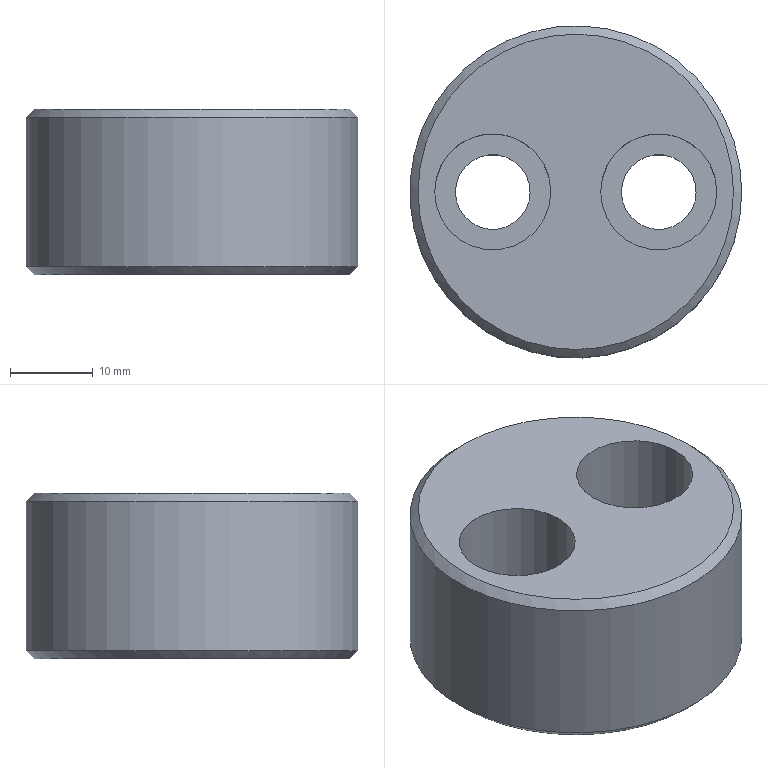Part | STEP file | 1_id2374_x_t | 1 solid | 11 faces | box 40 x 40 x 20 mm | volume 20116 mm3 | cylinder 5 | plane 4 | cone 2 | commonest cylinder face diameters 9 x2 14 x2 40 x1
STEP:
#1=CARTESIAN_POINT('',(0.,0.,0.));
#2=DIRECTION('',(0.,0.,1.));
#3=DIRECTION('',(1.,0.,0.));
#4=AXIS2_PLACEMENT_3D('',#1,#2,#3);
#5=CARTESIAN_POINT('',(78.5,0.813,59.));
#6=VERTEX_POINT('',#5);
#7=CARTESIAN_POINT('',(58.5,0.813,59.));
#8=DIRECTION('',(0.,0.,-1.));
#9=DIRECTION('',(1.,0.,0.));
#10=AXIS2_PLACEMENT_3D('',#7,#8,#9);
#11=CIRCLE('',#10,20.);
#12=CARTESIAN_POINT('',(58.5,0.813,-7.55));
#13=DIRECTION('',(0.,0.,1.));
#14=DIRECTION('',(1.,0.,0.));
#15=AXIS2_PLACEMENT_3D('',#12,#13,#14);
#16=CYLINDRICAL_SURFACE('',#15,20.);
#17=CARTESIAN_POINT('',(6.283,66.55));
#18=DIRECTION('',(-1.,0.));
#19=VECTOR('',#18,1.);
#20=LINE('',#17,#19);
#21=(GEOMETRIC_REPRESENTATION_CONTEXT(2)PARAMETRIC_REPRESENTATION_CONTEXT()REPRESENTATION_CONTEXT('',''));
#22=DEFINITIONAL_REPRESENTATION('',(#20),#21);
#23=PCURVE('',#16,#22);
#24=CARTESIAN_POINT('',(58.5,0.813,59.));
#25=DIRECTION('',(0.,0.,-1.));
#26=DIRECTION('',(1.,0.,0.));
#27=AXIS2_PLACEMENT_3D('',#24,#25,#26);
#28=CONICAL_SURFACE('',#27,20.,0.7854);
#29=CARTESIAN_POINT('',(0.,0.));
#30=DIRECTION('',(1.,0.));
#31=VECTOR('',#30,1.);
#32=LINE('',#29,#31);
#33=(GEOMETRIC_REPRESENTATION_CONTEXT(2)PARAMETRIC_REPRESENTATION_CONTEXT()REPRESENTATION_CONTEXT('',''));
#34=DEFINITIONAL_REPRESENTATION('',(#32),#33);
#35=PCURVE('',#28,#34);
#36=SURFACE_CURVE('',#11,(#23,#35),.PCURVE_S1.);
#37=EDGE_CURVE('',#6,#6,#36,.T.);
#38=ORIENTED_EDGE('',*,*,#37,.T.);
#39=CARTESIAN_POINT('',(78.5,0.813,41.));
#40=VERTEX_POINT('',#39);
#41=CARTESIAN_POINT('',(78.5,0.813,41.));
#42=CARTESIAN_POINT('',(78.5,0.813,59.));
#43=B_SPLINE_CURVE_WITH_KNOTS('',1,(#41,#42),.UNSPECIFIED.,.F.,.F.,(2,2),(48.55,66.55),.PIECEWISE_BEZIER_KNOTS.);
#44=CARTESIAN_POINT('',(0.,0.));
#45=DIRECTION('',(0.,1.));
#46=VECTOR('',#45,1.);
#47=LINE('',#44,#46);
#48=(GEOMETRIC_REPRESENTATION_CONTEXT(2)PARAMETRIC_REPRESENTATION_CONTEXT()REPRESENTATION_CONTEXT('',''));
#49=DEFINITIONAL_REPRESENTATION('',(#47),#48);
#50=PCURVE('',#16,#49);
#51=CARTESIAN_POINT('',(6.283,0.));
#52=DIRECTION('',(0.,1.));
#53=VECTOR('',#52,1.);
#54=LINE('',#51,#53);
#55=(GEOMETRIC_REPRESENTATION_CONTEXT(2)PARAMETRIC_REPRESENTATION_CONTEXT()REPRESENTATION_CONTEXT('',''));
#56=DEFINITIONAL_REPRESENTATION('',(#54),#55);
#57=PCURVE('',#16,#56);
#58=SEAM_CURVE('',#43,(#50,#57),.PCURVE_S1.);
#59=EDGE_CURVE('',#40,#6,#58,.T.);
#60=ORIENTED_EDGE('',*,*,#59,.F.);
#61=CARTESIAN_POINT('',(58.5,0.813,41.));
#62=DIRECTION('',(0.,0.,1.));
#63=DIRECTION('',(1.,0.,0.));
#64=AXIS2_PLACEMENT_3D('',#61,#62,#63);
#65=CIRCLE('',#64,20.);
#66=CARTESIAN_POINT('',(0.,48.55));
#67=DIRECTION('',(1.,0.));
#68=VECTOR('',#67,1.);
#69=LINE('',#66,#68);
#70=(GEOMETRIC_REPRESENTATION_CONTEXT(2)PARAMETRIC_REPRESENTATION_CONTEXT()REPRESENTATION_CONTEXT('',''));
#71=DEFINITIONAL_REPRESENTATION('',(#69),#70);
#72=PCURVE('',#16,#71);
#73=CARTESIAN_POINT('',(58.5,0.813,41.));
#74=DIRECTION('',(0.,0.,1.));
#75=DIRECTION('',(-1.,0.,0.));
#76=AXIS2_PLACEMENT_3D('',#73,#74,#75);
#77=CONICAL_SURFACE('',#76,20.,0.7854);
#78=CARTESIAN_POINT('',(3.142,0.));
#79=DIRECTION('',(1.,0.));
#80=VECTOR('',#79,1.);
#81=LINE('',#78,#80);
#82=(GEOMETRIC_REPRESENTATION_CONTEXT(2)PARAMETRIC_REPRESENTATION_CONTEXT()REPRESENTATION_CONTEXT('',''));
#83=DEFINITIONAL_REPRESENTATION('',(#81),#82);
#84=PCURVE('',#77,#83);
#85=SURFACE_CURVE('',#65,(#72,#84),.PCURVE_S1.);
#86=EDGE_CURVE('',#40,#40,#85,.T.);
#87=ORIENTED_EDGE('',*,*,#86,.T.);
#88=ORIENTED_EDGE('',*,*,#59,.T.);
#89=EDGE_LOOP('',(#38,#60,#87,#88));
#90=FACE_BOUND('',#89,.T.);
#91=ADVANCED_FACE('',(#90),#16,.T.);
#92=CARTESIAN_POINT('',(77.5,0.813,60.));
#93=VERTEX_POINT('',#92);
#94=CARTESIAN_POINT('',(58.5,0.813,60.));
#95=DIRECTION('',(0.,0.,1.));
#96=DIRECTION('',(1.,0.,0.));
#97=AXIS2_PLACEMENT_3D('',#94,#95,#96);
#98=CIRCLE('',#97,19.);
#99=CARTESIAN_POINT('',(58.5,0.813,60.));
#100=DIRECTION('',(0.,0.,1.));
#101=DIRECTION('',(1.,0.,0.));
#102=AXIS2_PLACEMENT_3D('',#99,#100,#101);
#103=PLANE('',#102);
#104=CARTESIAN_POINT('',(0.,0.));
#105=DIRECTION('',(1.,0.));
#106=AXIS2_PLACEMENT_2D('',#104,#105);
#107=CIRCLE('',#106,19.);
#108=(GEOMETRIC_REPRESENTATION_CONTEXT(2)PARAMETRIC_REPRESENTATION_CONTEXT()REPRESENTATION_CONTEXT('',''));
#109=DEFINITIONAL_REPRESENTATION('',(#107),#108);
#110=PCURVE('',#103,#109);
#111=CARTESIAN_POINT('',(6.283,-1.));
#112=DIRECTION('',(-1.,0.));
#113=VECTOR('',#112,1.);
#114=LINE('',#111,#113);
#115=(GEOMETRIC_REPRESENTATION_CONTEXT(2)PARAMETRIC_REPRESENTATION_CONTEXT()REPRESENTATION_CONTEXT('',''));
#116=DEFINITIONAL_REPRESENTATION('',(#114),#115);
#117=PCURVE('',#28,#116);
#118=SURFACE_CURVE('',#98,(#110,#117),.PCURVE_S1.);
#119=EDGE_CURVE('',#93,#93,#118,.T.);
#120=ORIENTED_EDGE('',*,*,#119,.T.);
#121=EDGE_LOOP('',(#120));
#122=FACE_BOUND('',#121,.T.);
#123=CARTESIAN_POINT('',(61.5,0.813,60.));
#124=VERTEX_POINT('',#123);
#125=CARTESIAN_POINT('',(68.5,0.813,60.));
#126=DIRECTION('',(0.,0.,-1.));
#127=DIRECTION('',(-1.,0.,0.));
#128=AXIS2_PLACEMENT_3D('',#125,#126,#127);
#129=CIRCLE('',#128,7.);
#130=CARTESIAN_POINT('',(3.,0.));
#131=CARTESIAN_POINT('',(3.,12.124));
#132=CARTESIAN_POINT('',(13.5,6.062));
#133=CARTESIAN_POINT('',(24.,0.));
#134=CARTESIAN_POINT('',(13.5,-6.062));
#135=CARTESIAN_POINT('',(3.,-12.124));
#136=CARTESIAN_POINT('',(3.,0.));
#137=(BOUNDED_CURVE()B_SPLINE_CURVE(2,(#130,#131,#132,#133,#134,#135,#136),.UNSPECIFIED.,.T.,.F.)B_SPLINE_CURVE_WITH_KNOTS((1,2,2,2,2,1),(-2.094,0.,2.094,4.189,6.283,8.378),.UNSPECIFIED.)CURVE()GEOMETRIC_REPRESENTATION_ITEM()RATIONAL_B_SPLINE_CURVE((1.,0.5,1.,0.5,1.,0.5,1.))REPRESENTATION_ITEM(''));
#138=(GEOMETRIC_REPRESENTATION_CONTEXT(2)PARAMETRIC_REPRESENTATION_CONTEXT()REPRESENTATION_CONTEXT('',''));
#139=DEFINITIONAL_REPRESENTATION('',(#137),#138);
#140=PCURVE('',#103,#139);
#141=CARTESIAN_POINT('',(68.5,0.813,27.45));
#142=DIRECTION('',(0.,0.,1.));
#143=DIRECTION('',(1.,0.,0.));
#144=AXIS2_PLACEMENT_3D('',#141,#142,#143);
#145=CYLINDRICAL_SURFACE('',#144,7.);
#146=CARTESIAN_POINT('',(9.425,32.55));
#147=DIRECTION('',(-1.,0.));
#148=VECTOR('',#147,1.);
#149=LINE('',#146,#148);
#150=(GEOMETRIC_REPRESENTATION_CONTEXT(2)PARAMETRIC_REPRESENTATION_CONTEXT()REPRESENTATION_CONTEXT('',''));
#151=DEFINITIONAL_REPRESENTATION('',(#149),#150);
#152=PCURVE('',#145,#151);
#153=SURFACE_CURVE('',#129,(#140,#152),.PCURVE_S1.);
#154=EDGE_CURVE('',#124,#124,#153,.T.);
#155=ORIENTED_EDGE('',*,*,#154,.T.);
#156=EDGE_LOOP('',(#155));
#157=FACE_BOUND('',#156,.T.);
#158=CARTESIAN_POINT('',(41.5,0.813,60.));
#159=VERTEX_POINT('',#158);
#160=CARTESIAN_POINT('',(48.5,0.813,60.));
#161=DIRECTION('',(0.,0.,1.));
#162=DIRECTION('',(-1.,0.,0.));
#163=AXIS2_PLACEMENT_3D('',#160,#161,#162);
#164=CIRCLE('',#163,7.);
#165=CARTESIAN_POINT('',(-10.,0.));
#166=DIRECTION('',(-1.,0.));
#167=AXIS2_PLACEMENT_2D('',#165,#166);
#168=CIRCLE('',#167,7.);
#169=(GEOMETRIC_REPRESENTATION_CONTEXT(2)PARAMETRIC_REPRESENTATION_CONTEXT()REPRESENTATION_CONTEXT('',''));
#170=DEFINITIONAL_REPRESENTATION('',(#168),#169);
#171=PCURVE('',#103,#170);
#172=CARTESIAN_POINT('',(48.5,0.813,27.45));
#173=DIRECTION('',(0.,0.,1.));
#174=DIRECTION('',(1.,0.,0.));
#175=AXIS2_PLACEMENT_3D('',#172,#173,#174);
#176=CYLINDRICAL_SURFACE('',#175,7.);
#177=CARTESIAN_POINT('',(3.142,32.55));
#178=DIRECTION('',(1.,0.));
#179=VECTOR('',#178,1.);
#180=LINE('',#177,#179);
#181=(GEOMETRIC_REPRESENTATION_CONTEXT(2)PARAMETRIC_REPRESENTATION_CONTEXT()REPRESENTATION_CONTEXT('',''));
#182=DEFINITIONAL_REPRESENTATION('',(#180),#181);
#183=PCURVE('',#176,#182);
#184=SURFACE_CURVE('',#164,(#171,#183),.PCURVE_S1.);
#185=EDGE_CURVE('',#159,#159,#184,.T.);
#186=ORIENTED_EDGE('',*,*,#185,.F.);
#187=EDGE_LOOP('',(#186));
#188=FACE_BOUND('',#187,.T.);
#189=ADVANCED_FACE('',(#122,#157,#188),#103,.T.);
#190=CARTESIAN_POINT('',(41.5,0.813,47.));
#191=VERTEX_POINT('',#190);
#192=CARTESIAN_POINT('',(48.5,0.813,47.));
#193=DIRECTION('',(0.,0.,-1.));
#194=DIRECTION('',(-1.,0.,0.));
#195=AXIS2_PLACEMENT_3D('',#192,#193,#194);
#196=CIRCLE('',#195,7.);
#197=CARTESIAN_POINT('',(63.5,0.813,47.));
#198=DIRECTION('',(0.,0.,1.));
#199=DIRECTION('',(1.,0.,0.));
#200=AXIS2_PLACEMENT_3D('',#197,#198,#199);
#201=PLANE('',#200);
#202=CARTESIAN_POINT('',(-22.,0.));
#203=CARTESIAN_POINT('',(-22.,12.124));
#204=CARTESIAN_POINT('',(-11.5,6.062));
#205=CARTESIAN_POINT('',(-1.,0.));
#206=CARTESIAN_POINT('',(-11.5,-6.062));
#207=CARTESIAN_POINT('',(-22.,-12.124));
#208=CARTESIAN_POINT('',(-22.,0.));
#209=(BOUNDED_CURVE()B_SPLINE_CURVE(2,(#202,#203,#204,#205,#206,#207,#208),.UNSPECIFIED.,.T.,.F.)B_SPLINE_CURVE_WITH_KNOTS((1,2,2,2,2,1),(-2.094,0.,2.094,4.189,6.283,8.378),.UNSPECIFIED.)CURVE()GEOMETRIC_REPRESENTATION_ITEM()RATIONAL_B_SPLINE_CURVE((1.,0.5,1.,0.5,1.,0.5,1.))REPRESENTATION_ITEM(''));
#210=(GEOMETRIC_REPRESENTATION_CONTEXT(2)PARAMETRIC_REPRESENTATION_CONTEXT()REPRESENTATION_CONTEXT('',''));
#211=DEFINITIONAL_REPRESENTATION('',(#209),#210);
#212=PCURVE('',#201,#211);
#213=CARTESIAN_POINT('',(9.425,19.55));
#214=DIRECTION('',(-1.,0.));
#215=VECTOR('',#214,1.);
#216=LINE('',#213,#215);
#217=(GEOMETRIC_REPRESENTATION_CONTEXT(2)PARAMETRIC_REPRESENTATION_CONTEXT()REPRESENTATION_CONTEXT('',''));
#218=DEFINITIONAL_REPRESENTATION('',(#216),#217);
#219=PCURVE('',#176,#218);
#220=SURFACE_CURVE('',#196,(#212,#219),.PCURVE_S1.);
#221=EDGE_CURVE('',#191,#191,#220,.T.);
#222=ORIENTED_EDGE('',*,*,#221,.F.);
#223=EDGE_LOOP('',(#222));
#224=FACE_BOUND('',#223,.T.);
#225=CARTESIAN_POINT('',(44.,0.813,47.));
#226=VERTEX_POINT('',#225);
#227=CARTESIAN_POINT('',(48.5,0.813,47.));
#228=DIRECTION('',(0.,0.,-1.));
#229=DIRECTION('',(-1.,0.,0.));
#230=AXIS2_PLACEMENT_3D('',#227,#228,#229);
#231=CIRCLE('',#230,4.5);
#232=CARTESIAN_POINT('',(-19.5,0.));
#233=CARTESIAN_POINT('',(-19.5,7.794));
#234=CARTESIAN_POINT('',(-12.75,3.897));
#235=CARTESIAN_POINT('',(-6.,0.));
#236=CARTESIAN_POINT('',(-12.75,-3.897));
#237=CARTESIAN_POINT('',(-19.5,-7.794));
#238=CARTESIAN_POINT('',(-19.5,0.));
#239=(BOUNDED_CURVE()B_SPLINE_CURVE(2,(#232,#233,#234,#235,#236,#237,#238),.UNSPECIFIED.,.T.,.F.)B_SPLINE_CURVE_WITH_KNOTS((1,2,2,2,2,1),(-2.094,0.,2.094,4.189,6.283,8.378),.UNSPECIFIED.)CURVE()GEOMETRIC_REPRESENTATION_ITEM()RATIONAL_B_SPLINE_CURVE((1.,0.5,1.,0.5,1.,0.5,1.))REPRESENTATION_ITEM(''));
#240=(GEOMETRIC_REPRESENTATION_CONTEXT(2)PARAMETRIC_REPRESENTATION_CONTEXT()REPRESENTATION_CONTEXT('',''));
#241=DEFINITIONAL_REPRESENTATION('',(#239),#240);
#242=PCURVE('',#201,#241);
#243=CARTESIAN_POINT('',(48.5,0.813,128.5));
#244=DIRECTION('',(0.,0.,-1.));
#245=DIRECTION('',(1.,0.,0.));
#246=AXIS2_PLACEMENT_3D('',#243,#244,#245);
#247=CYLINDRICAL_SURFACE('',#246,4.5);
#248=CARTESIAN_POINT('',(3.142,81.5));
#249=DIRECTION('',(1.,0.));
#250=VECTOR('',#249,1.);
#251=LINE('',#248,#250);
#252=(GEOMETRIC_REPRESENTATION_CONTEXT(2)PARAMETRIC_REPRESENTATION_CONTEXT()REPRESENTATION_CONTEXT('',''));
#253=DEFINITIONAL_REPRESENTATION('',(#251),#252);
#254=PCURVE('',#247,#253);
#255=SURFACE_CURVE('',#231,(#242,#254),.PCURVE_S1.);
#256=EDGE_CURVE('',#226,#226,#255,.T.);
#257=ORIENTED_EDGE('',*,*,#256,.T.);
#258=EDGE_LOOP('',(#257));
#259=FACE_BOUND('',#258,.T.);
#260=ADVANCED_FACE('',(#224,#259),#201,.T.);
#261=CARTESIAN_POINT('',(44.,0.813,40.));
#262=VERTEX_POINT('',#261);
#263=CARTESIAN_POINT('',(48.5,0.813,40.));
#264=DIRECTION('',(0.,0.,1.));
#265=DIRECTION('',(-1.,0.,0.));
#266=AXIS2_PLACEMENT_3D('',#263,#264,#265);
#267=CIRCLE('',#266,4.5);
#268=CARTESIAN_POINT('',(9.425,88.5));
#269=DIRECTION('',(-1.,0.));
#270=VECTOR('',#269,1.);
#271=LINE('',#268,#270);
#272=(GEOMETRIC_REPRESENTATION_CONTEXT(2)PARAMETRIC_REPRESENTATION_CONTEXT()REPRESENTATION_CONTEXT('',''));
#273=DEFINITIONAL_REPRESENTATION('',(#271),#272);
#274=PCURVE('',#247,#273);
#275=CARTESIAN_POINT('',(-254.,130.813,40.));
#276=DIRECTION('',(0.,0.,1.));
#277=DIRECTION('',(1.,0.,0.));
#278=AXIS2_PLACEMENT_3D('',#275,#276,#277);
#279=PLANE('',#278);
#280=CARTESIAN_POINT('',(302.5,-130.));
#281=DIRECTION('',(-1.,0.));
#282=AXIS2_PLACEMENT_2D('',#280,#281);
#283=CIRCLE('',#282,4.5);
#284=(GEOMETRIC_REPRESENTATION_CONTEXT(2)PARAMETRIC_REPRESENTATION_CONTEXT()REPRESENTATION_CONTEXT('',''));
#285=DEFINITIONAL_REPRESENTATION('',(#283),#284);
#286=PCURVE('',#279,#285);
#287=SURFACE_CURVE('',#267,(#274,#286),.PCURVE_S1.);
#288=EDGE_CURVE('',#262,#262,#287,.T.);
#289=ORIENTED_EDGE('',*,*,#288,.T.);
#290=CARTESIAN_POINT('',(44.,0.813,47.));
#291=CARTESIAN_POINT('',(44.,0.813,40.));
#292=B_SPLINE_CURVE_WITH_KNOTS('',1,(#290,#291),.UNSPECIFIED.,.F.,.F.,(2,2),(81.5,88.5),.PIECEWISE_BEZIER_KNOTS.);
#293=CARTESIAN_POINT('',(3.142,0.));
#294=DIRECTION('',(0.,1.));
#295=VECTOR('',#294,1.);
#296=LINE('',#293,#295);
#297=(GEOMETRIC_REPRESENTATION_CONTEXT(2)PARAMETRIC_REPRESENTATION_CONTEXT()REPRESENTATION_CONTEXT('',''));
#298=DEFINITIONAL_REPRESENTATION('',(#296),#297);
#299=PCURVE('',#247,#298);
#300=CARTESIAN_POINT('',(9.425,0.));
#301=DIRECTION('',(0.,1.));
#302=VECTOR('',#301,1.);
#303=LINE('',#300,#302);
#304=(GEOMETRIC_REPRESENTATION_CONTEXT(2)PARAMETRIC_REPRESENTATION_CONTEXT()REPRESENTATION_CONTEXT('',''));
#305=DEFINITIONAL_REPRESENTATION('',(#303),#304);
#306=PCURVE('',#247,#305);
#307=SEAM_CURVE('',#292,(#299,#306),.PCURVE_S1.);
#308=EDGE_CURVE('',#226,#262,#307,.T.);
#309=ORIENTED_EDGE('',*,*,#308,.F.);
#310=ORIENTED_EDGE('',*,*,#256,.T.);
#311=ORIENTED_EDGE('',*,*,#308,.T.);
#312=EDGE_LOOP('',(#289,#309,#310,#311));
#313=FACE_BOUND('',#312,.F.);
#314=ADVANCED_FACE('',(#313),#247,.F.);
#315=ORIENTED_EDGE('',*,*,#185,.F.);
#316=CARTESIAN_POINT('',(41.5,0.813,47.));
#317=CARTESIAN_POINT('',(41.5,0.813,60.));
#318=B_SPLINE_CURVE_WITH_KNOTS('',1,(#316,#317),.UNSPECIFIED.,.F.,.F.,(2,2),(19.55,32.55),.PIECEWISE_BEZIER_KNOTS.);
#319=CARTESIAN_POINT('',(3.142,0.));
#320=DIRECTION('',(0.,1.));
#321=VECTOR('',#320,1.);
#322=LINE('',#319,#321);
#323=(GEOMETRIC_REPRESENTATION_CONTEXT(2)PARAMETRIC_REPRESENTATION_CONTEXT()REPRESENTATION_CONTEXT('',''));
#324=DEFINITIONAL_REPRESENTATION('',(#322),#323);
#325=PCURVE('',#176,#324);
#326=CARTESIAN_POINT('',(9.425,0.));
#327=DIRECTION('',(0.,1.));
#328=VECTOR('',#327,1.);
#329=LINE('',#326,#328);
#330=(GEOMETRIC_REPRESENTATION_CONTEXT(2)PARAMETRIC_REPRESENTATION_CONTEXT()REPRESENTATION_CONTEXT('',''));
#331=DEFINITIONAL_REPRESENTATION('',(#329),#330);
#332=PCURVE('',#176,#331);
#333=SEAM_CURVE('',#318,(#325,#332),.PCURVE_S1.);
#334=EDGE_CURVE('',#191,#159,#333,.T.);
#335=ORIENTED_EDGE('',*,*,#334,.F.);
#336=ORIENTED_EDGE('',*,*,#221,.F.);
#337=ORIENTED_EDGE('',*,*,#334,.T.);
#338=EDGE_LOOP('',(#315,#335,#336,#337));
#339=FACE_BOUND('',#338,.F.);
#340=ADVANCED_FACE('',(#339),#176,.F.);
#341=CARTESIAN_POINT('',(61.5,0.813,47.));
#342=VERTEX_POINT('',#341);
#343=CARTESIAN_POINT('',(68.5,0.813,47.));
#344=DIRECTION('',(0.,0.,-1.));
#345=DIRECTION('',(-1.,0.,0.));
#346=AXIS2_PLACEMENT_3D('',#343,#344,#345);
#347=CIRCLE('',#346,7.);
#348=CARTESIAN_POINT('',(53.5,0.813,47.));
#349=DIRECTION('',(0.,0.,1.));
#350=DIRECTION('',(1.,0.,0.));
#351=AXIS2_PLACEMENT_3D('',#348,#349,#350);
#352=PLANE('',#351);
#353=CARTESIAN_POINT('',(8.,0.));
#354=CARTESIAN_POINT('',(8.,12.124));
#355=CARTESIAN_POINT('',(18.5,6.062));
#356=CARTESIAN_POINT('',(29.,0.));
#357=CARTESIAN_POINT('',(18.5,-6.062));
#358=CARTESIAN_POINT('',(8.,-12.124));
#359=CARTESIAN_POINT('',(8.,0.));
#360=(BOUNDED_CURVE()B_SPLINE_CURVE(2,(#353,#354,#355,#356,#357,#358,#359),.UNSPECIFIED.,.T.,.F.)B_SPLINE_CURVE_WITH_KNOTS((1,2,2,2,2,1),(-2.094,0.,2.094,4.189,6.283,8.378),.UNSPECIFIED.)CURVE()GEOMETRIC_REPRESENTATION_ITEM()RATIONAL_B_SPLINE_CURVE((1.,0.5,1.,0.5,1.,0.5,1.))REPRESENTATION_ITEM(''));
#361=(GEOMETRIC_REPRESENTATION_CONTEXT(2)PARAMETRIC_REPRESENTATION_CONTEXT()REPRESENTATION_CONTEXT('',''));
#362=DEFINITIONAL_REPRESENTATION('',(#360),#361);
#363=PCURVE('',#352,#362);
#364=CARTESIAN_POINT('',(9.425,19.55));
#365=DIRECTION('',(-1.,0.));
#366=VECTOR('',#365,1.);
#367=LINE('',#364,#366);
#368=(GEOMETRIC_REPRESENTATION_CONTEXT(2)PARAMETRIC_REPRESENTATION_CONTEXT()REPRESENTATION_CONTEXT('',''));
#369=DEFINITIONAL_REPRESENTATION('',(#367),#368);
#370=PCURVE('',#145,#369);
#371=SURFACE_CURVE('',#347,(#363,#370),.PCURVE_S1.);
#372=EDGE_CURVE('',#342,#342,#371,.T.);
#373=ORIENTED_EDGE('',*,*,#372,.F.);
#374=EDGE_LOOP('',(#373));
#375=FACE_BOUND('',#374,.T.);
#376=CARTESIAN_POINT('',(64.,0.813,47.));
#377=VERTEX_POINT('',#376);
#378=CARTESIAN_POINT('',(68.5,0.813,47.));
#379=DIRECTION('',(0.,0.,-1.));
#380=DIRECTION('',(-1.,0.,0.));
#381=AXIS2_PLACEMENT_3D('',#378,#379,#380);
#382=CIRCLE('',#381,4.5);
#383=CARTESIAN_POINT('',(10.5,0.));
#384=CARTESIAN_POINT('',(10.5,7.794));
#385=CARTESIAN_POINT('',(17.25,3.897));
#386=CARTESIAN_POINT('',(24.,0.));
#387=CARTESIAN_POINT('',(17.25,-3.897));
#388=CARTESIAN_POINT('',(10.5,-7.794));
#389=CARTESIAN_POINT('',(10.5,0.));
#390=(BOUNDED_CURVE()B_SPLINE_CURVE(2,(#383,#384,#385,#386,#387,#388,#389),.UNSPECIFIED.,.T.,.F.)B_SPLINE_CURVE_WITH_KNOTS((1,2,2,2,2,1),(-2.094,0.,2.094,4.189,6.283,8.378),.UNSPECIFIED.)CURVE()GEOMETRIC_REPRESENTATION_ITEM()RATIONAL_B_SPLINE_CURVE((1.,0.5,1.,0.5,1.,0.5,1.))REPRESENTATION_ITEM(''));
#391=(GEOMETRIC_REPRESENTATION_CONTEXT(2)PARAMETRIC_REPRESENTATION_CONTEXT()REPRESENTATION_CONTEXT('',''));
#392=DEFINITIONAL_REPRESENTATION('',(#390),#391);
#393=PCURVE('',#352,#392);
#394=CARTESIAN_POINT('',(68.5,0.813,128.5));
#395=DIRECTION('',(0.,0.,-1.));
#396=DIRECTION('',(1.,0.,0.));
#397=AXIS2_PLACEMENT_3D('',#394,#395,#396);
#398=CYLINDRICAL_SURFACE('',#397,4.5);
#399=CARTESIAN_POINT('',(3.142,81.5));
#400=DIRECTION('',(1.,0.));
#401=VECTOR('',#400,1.);
#402=LINE('',#399,#401);
#403=(GEOMETRIC_REPRESENTATION_CONTEXT(2)PARAMETRIC_REPRESENTATION_CONTEXT()REPRESENTATION_CONTEXT('',''));
#404=DEFINITIONAL_REPRESENTATION('',(#402),#403);
#405=PCURVE('',#398,#404);
#406=SURFACE_CURVE('',#382,(#393,#405),.PCURVE_S1.);
#407=EDGE_CURVE('',#377,#377,#406,.T.);
#408=ORIENTED_EDGE('',*,*,#407,.T.);
#409=EDGE_LOOP('',(#408));
#410=FACE_BOUND('',#409,.T.);
#411=ADVANCED_FACE('',(#375,#410),#352,.T.);
#412=ORIENTED_EDGE('',*,*,#154,.T.);
#413=CARTESIAN_POINT('',(61.5,0.813,47.));
#414=CARTESIAN_POINT('',(61.5,0.813,60.));
#415=B_SPLINE_CURVE_WITH_KNOTS('',1,(#413,#414),.UNSPECIFIED.,.F.,.F.,(2,2),(19.55,32.55),.PIECEWISE_BEZIER_KNOTS.);
#416=CARTESIAN_POINT('',(3.142,0.));
#417=DIRECTION('',(0.,1.));
#418=VECTOR('',#417,1.);
#419=LINE('',#416,#418);
#420=(GEOMETRIC_REPRESENTATION_CONTEXT(2)PARAMETRIC_REPRESENTATION_CONTEXT()REPRESENTATION_CONTEXT('',''));
#421=DEFINITIONAL_REPRESENTATION('',(#419),#420);
#422=PCURVE('',#145,#421);
#423=CARTESIAN_POINT('',(9.425,0.));
#424=DIRECTION('',(0.,1.));
#425=VECTOR('',#424,1.);
#426=LINE('',#423,#425);
#427=(GEOMETRIC_REPRESENTATION_CONTEXT(2)PARAMETRIC_REPRESENTATION_CONTEXT()REPRESENTATION_CONTEXT('',''));
#428=DEFINITIONAL_REPRESENTATION('',(#426),#427);
#429=PCURVE('',#145,#428);
#430=SEAM_CURVE('',#415,(#422,#429),.PCURVE_S1.);
#431=EDGE_CURVE('',#342,#124,#430,.T.);
#432=ORIENTED_EDGE('',*,*,#431,.F.);
#433=ORIENTED_EDGE('',*,*,#372,.F.);
#434=ORIENTED_EDGE('',*,*,#431,.T.);
#435=EDGE_LOOP('',(#412,#432,#433,#434));
#436=FACE_BOUND('',#435,.F.);
#437=ADVANCED_FACE('',(#436),#145,.F.);
#438=CARTESIAN_POINT('',(64.,0.813,40.));
#439=VERTEX_POINT('',#438);
#440=CARTESIAN_POINT('',(68.5,0.813,40.));
#441=DIRECTION('',(0.,0.,-1.));
#442=DIRECTION('',(-1.,0.,0.));
#443=AXIS2_PLACEMENT_3D('',#440,#441,#442);
#444=CIRCLE('',#443,4.5);
#445=CARTESIAN_POINT('',(3.142,88.5));
#446=DIRECTION('',(1.,0.));
#447=VECTOR('',#446,1.);
#448=LINE('',#445,#447);
#449=(GEOMETRIC_REPRESENTATION_CONTEXT(2)PARAMETRIC_REPRESENTATION_CONTEXT()REPRESENTATION_CONTEXT('',''));
#450=DEFINITIONAL_REPRESENTATION('',(#448),#449);
#451=PCURVE('',#398,#450);
#452=CARTESIAN_POINT('',(318.,-130.));
#453=CARTESIAN_POINT('',(318.,-122.206));
#454=CARTESIAN_POINT('',(324.75,-126.103));
#455=CARTESIAN_POINT('',(331.5,-130.));
#456=CARTESIAN_POINT('',(324.75,-133.897));
#457=CARTESIAN_POINT('',(318.,-137.794));
#458=CARTESIAN_POINT('',(318.,-130.));
#459=(BOUNDED_CURVE()B_SPLINE_CURVE(2,(#452,#453,#454,#455,#456,#457,#458),.UNSPECIFIED.,.T.,.F.)B_SPLINE_CURVE_WITH_KNOTS((1,2,2,2,2,1),(-2.094,0.,2.094,4.189,6.283,8.378),.UNSPECIFIED.)CURVE()GEOMETRIC_REPRESENTATION_ITEM()RATIONAL_B_SPLINE_CURVE((1.,0.5,1.,0.5,1.,0.5,1.))REPRESENTATION_ITEM(''));
#460=(GEOMETRIC_REPRESENTATION_CONTEXT(2)PARAMETRIC_REPRESENTATION_CONTEXT()REPRESENTATION_CONTEXT('',''));
#461=DEFINITIONAL_REPRESENTATION('',(#459),#460);
#462=PCURVE('',#279,#461);
#463=SURFACE_CURVE('',#444,(#451,#462),.PCURVE_S1.);
#464=EDGE_CURVE('',#439,#439,#463,.T.);
#465=ORIENTED_EDGE('',*,*,#464,.F.);
#466=CARTESIAN_POINT('',(64.,0.813,47.));
#467=CARTESIAN_POINT('',(64.,0.813,40.));
#468=B_SPLINE_CURVE_WITH_KNOTS('',1,(#466,#467),.UNSPECIFIED.,.F.,.F.,(2,2),(81.5,88.5),.PIECEWISE_BEZIER_KNOTS.);
#469=CARTESIAN_POINT('',(3.142,0.));
#470=DIRECTION('',(0.,1.));
#471=VECTOR('',#470,1.);
#472=LINE('',#469,#471);
#473=(GEOMETRIC_REPRESENTATION_CONTEXT(2)PARAMETRIC_REPRESENTATION_CONTEXT()REPRESENTATION_CONTEXT('',''));
#474=DEFINITIONAL_REPRESENTATION('',(#472),#473);
#475=PCURVE('',#398,#474);
#476=CARTESIAN_POINT('',(9.425,0.));
#477=DIRECTION('',(0.,1.));
#478=VECTOR('',#477,1.);
#479=LINE('',#476,#478);
#480=(GEOMETRIC_REPRESENTATION_CONTEXT(2)PARAMETRIC_REPRESENTATION_CONTEXT()REPRESENTATION_CONTEXT('',''));
#481=DEFINITIONAL_REPRESENTATION('',(#479),#480);
#482=PCURVE('',#398,#481);
#483=SEAM_CURVE('',#468,(#475,#482),.PCURVE_S1.);
#484=EDGE_CURVE('',#377,#439,#483,.T.);
#485=ORIENTED_EDGE('',*,*,#484,.F.);
#486=ORIENTED_EDGE('',*,*,#407,.T.);
#487=ORIENTED_EDGE('',*,*,#484,.T.);
#488=EDGE_LOOP('',(#465,#485,#486,#487));
#489=FACE_BOUND('',#488,.F.);
#490=ADVANCED_FACE('',(#489),#398,.F.);
#491=CARTESIAN_POINT('',(77.5,0.813,40.));
#492=VERTEX_POINT('',#491);
#493=CARTESIAN_POINT('',(58.5,0.813,40.));
#494=DIRECTION('',(0.,0.,-1.));
#495=DIRECTION('',(1.,0.,0.));
#496=AXIS2_PLACEMENT_3D('',#493,#494,#495);
#497=CIRCLE('',#496,19.);
#498=CARTESIAN_POINT('',(331.5,-130.));
#499=CARTESIAN_POINT('',(331.5,-162.909));
#500=CARTESIAN_POINT('',(303.,-146.454));
#501=CARTESIAN_POINT('',(274.5,-130.));
#502=CARTESIAN_POINT('',(303.,-113.546));
#503=CARTESIAN_POINT('',(331.5,-97.091));
#504=CARTESIAN_POINT('',(331.5,-130.));
#505=(BOUNDED_CURVE()B_SPLINE_CURVE(2,(#498,#499,#500,#501,#502,#503,#504),.UNSPECIFIED.,.T.,.F.)B_SPLINE_CURVE_WITH_KNOTS((1,2,2,2,2,1),(-2.094,0.,2.094,4.189,6.283,8.378),.UNSPECIFIED.)CURVE()GEOMETRIC_REPRESENTATION_ITEM()RATIONAL_B_SPLINE_CURVE((1.,0.5,1.,0.5,1.,0.5,1.))REPRESENTATION_ITEM(''));
#506=(GEOMETRIC_REPRESENTATION_CONTEXT(2)PARAMETRIC_REPRESENTATION_CONTEXT()REPRESENTATION_CONTEXT('',''));
#507=DEFINITIONAL_REPRESENTATION('',(#505),#506);
#508=PCURVE('',#279,#507);
#509=CARTESIAN_POINT('',(9.425,-1.));
#510=DIRECTION('',(-1.,0.));
#511=VECTOR('',#510,1.);
#512=LINE('',#509,#511);
#513=(GEOMETRIC_REPRESENTATION_CONTEXT(2)PARAMETRIC_REPRESENTATION_CONTEXT()REPRESENTATION_CONTEXT('',''));
#514=DEFINITIONAL_REPRESENTATION('',(#512),#513);
#515=PCURVE('',#77,#514);
#516=SURFACE_CURVE('',#497,(#508,#515),.PCURVE_S1.);
#517=EDGE_CURVE('',#492,#492,#516,.T.);
#518=ORIENTED_EDGE('',*,*,#517,.T.);
#519=EDGE_LOOP('',(#518));
#520=FACE_BOUND('',#519,.T.);
#521=ORIENTED_EDGE('',*,*,#288,.T.);
#522=EDGE_LOOP('',(#521));
#523=FACE_BOUND('',#522,.T.);
#524=ORIENTED_EDGE('',*,*,#464,.F.);
#525=EDGE_LOOP('',(#524));
#526=FACE_BOUND('',#525,.T.);
#527=ADVANCED_FACE('',(#520,#523,#526),#279,.F.);
#528=ORIENTED_EDGE('',*,*,#119,.F.);
#529=CARTESIAN_POINT('',(77.5,0.813,60.));
#530=CARTESIAN_POINT('',(78.5,0.813,59.));
#531=B_SPLINE_CURVE_WITH_KNOTS('',1,(#529,#530),.UNSPECIFIED.,.F.,.F.,(2,2),(-1.414,0.),.PIECEWISE_BEZIER_KNOTS.);
#532=CARTESIAN_POINT('',(6.283,0.));
#533=DIRECTION('',(0.,1.));
#534=VECTOR('',#533,1.);
#535=LINE('',#532,#534);
#536=(GEOMETRIC_REPRESENTATION_CONTEXT(2)PARAMETRIC_REPRESENTATION_CONTEXT()REPRESENTATION_CONTEXT('',''));
#537=DEFINITIONAL_REPRESENTATION('',(#535),#536);
#538=PCURVE('',#28,#537);
#539=CARTESIAN_POINT('',(0.,0.));
#540=DIRECTION('',(0.,1.));
#541=VECTOR('',#540,1.);
#542=LINE('',#539,#541);
#543=(GEOMETRIC_REPRESENTATION_CONTEXT(2)PARAMETRIC_REPRESENTATION_CONTEXT()REPRESENTATION_CONTEXT('',''));
#544=DEFINITIONAL_REPRESENTATION('',(#542),#543);
#545=PCURVE('',#28,#544);
#546=SEAM_CURVE('',#531,(#538,#545),.PCURVE_S1.);
#547=EDGE_CURVE('',#93,#6,#546,.T.);
#548=ORIENTED_EDGE('',*,*,#547,.T.);
#549=ORIENTED_EDGE('',*,*,#37,.F.);
#550=ORIENTED_EDGE('',*,*,#547,.F.);
#551=EDGE_LOOP('',(#528,#548,#549,#550));
#552=FACE_BOUND('',#551,.T.);
#553=ADVANCED_FACE('',(#552),#28,.T.);
#554=ORIENTED_EDGE('',*,*,#517,.F.);
#555=CARTESIAN_POINT('',(77.5,0.813,40.));
#556=CARTESIAN_POINT('',(78.5,0.813,41.));
#557=B_SPLINE_CURVE_WITH_KNOTS('',1,(#555,#556),.UNSPECIFIED.,.F.,.F.,(2,2),(-1.414,0.),.PIECEWISE_BEZIER_KNOTS.);
#558=CARTESIAN_POINT('',(9.425,0.));
#559=DIRECTION('',(0.,1.));
#560=VECTOR('',#559,1.);
#561=LINE('',#558,#560);
#562=(GEOMETRIC_REPRESENTATION_CONTEXT(2)PARAMETRIC_REPRESENTATION_CONTEXT()REPRESENTATION_CONTEXT('',''));
#563=DEFINITIONAL_REPRESENTATION('',(#561),#562);
#564=PCURVE('',#77,#563);
#565=CARTESIAN_POINT('',(3.142,0.));
#566=DIRECTION('',(0.,1.));
#567=VECTOR('',#566,1.);
#568=LINE('',#565,#567);
#569=(GEOMETRIC_REPRESENTATION_CONTEXT(2)PARAMETRIC_REPRESENTATION_CONTEXT()REPRESENTATION_CONTEXT('',''));
#570=DEFINITIONAL_REPRESENTATION('',(#568),#569);
#571=PCURVE('',#77,#570);
#572=SEAM_CURVE('',#557,(#564,#571),.PCURVE_S1.);
#573=EDGE_CURVE('',#492,#40,#572,.T.);
#574=ORIENTED_EDGE('',*,*,#573,.T.);
#575=ORIENTED_EDGE('',*,*,#86,.F.);
#576=ORIENTED_EDGE('',*,*,#573,.F.);
#577=EDGE_LOOP('',(#554,#574,#575,#576));
#578=FACE_BOUND('',#577,.T.);
#579=ADVANCED_FACE('',(#578),#77,.T.);
#580=CLOSED_SHELL('',(#91,#189,#260,#314,#340,#411,#437,#490,#527,#553,#579));
#581=MANIFOLD_SOLID_BREP('',#580);
#582=(LENGTH_UNIT()NAMED_UNIT(*)SI_UNIT(.MILLI.,.METRE.));
#583=UNCERTAINTY_MEASURE_WITH_UNIT(LENGTH_MEASURE(0.00001),#582,'','');
#584=(NAMED_UNIT(*)PLANE_ANGLE_UNIT()SI_UNIT($,.RADIAN.));
#585=(NAMED_UNIT(*)SI_UNIT($,.STERADIAN.)SOLID_ANGLE_UNIT());
#586=(GEOMETRIC_REPRESENTATION_CONTEXT(3)GLOBAL_UNCERTAINTY_ASSIGNED_CONTEXT((#583))GLOBAL_UNIT_ASSIGNED_CONTEXT((#582,#584,#585))REPRESENTATION_CONTEXT('',''));
#587=ADVANCED_BREP_SHAPE_REPRESENTATION('',(#4,#581),#586);